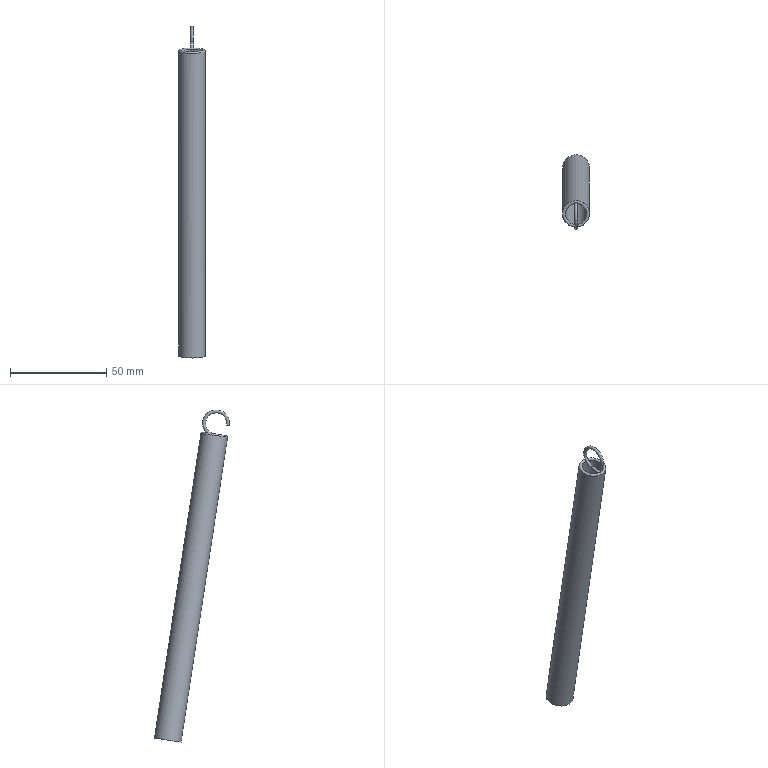Part | NX | features 1 2 | 1 solid | 7 faces | box 14 x 39.013 x 172.675 mm | volume 9539 mm3 | cylinder 3 | plane 2 | torus 2 | commonest cylinder face diameters 1.5 x1 11 x1 14 x1
STEP:
#1=CARTESIAN_POINT('',(-24.935,47.341,-652.78));
#2=VERTEX_POINT('',#1);
#3=CARTESIAN_POINT('',(-24.935,46.602,-652.906));
#4=DIRECTION('',(0.,0.1679,-0.9858));
#5=DIRECTION('',(0.,0.9858,0.1679));
#6=AXIS2_PLACEMENT_3D('',#3,#4,#5);
#7=CIRCLE('',#6,0.75);
#8=EDGE_CURVE('',#2,#2,#7,.F.);
#9=ORIENTED_EDGE('',*,*,#8,.F.);
#10=EDGE_LOOP('',(#9));
#11=FACE_BOUND('',#10,.T.);
#12=CARTESIAN_POINT('',(-24.935,46.602,-652.906));
#13=DIRECTION('',(0.,0.1679,-0.9858));
#14=DIRECTION('',(0.,-0.9858,-0.1679));
#15=AXIS2_PLACEMENT_3D('',#12,#13,#14);
#16=PLANE('',#15);
#17=ADVANCED_FACE('',(#11),#16,.T.);
#18=CARTESIAN_POINT('',(-25.685,53.704,-658.036));
#19=VERTEX_POINT('',#18);
#20=CARTESIAN_POINT('',(-24.935,53.704,-658.036));
#21=DIRECTION('',(0.,-0.9886,-0.1507));
#22=DIRECTION('',(-1.,0.,0.));
#23=AXIS2_PLACEMENT_3D('',#20,#21,#22);
#24=CIRCLE('',#23,0.75);
#25=EDGE_CURVE('',#19,#19,#24,.T.);
#26=ORIENTED_EDGE('',*,*,#25,.F.);
#27=EDGE_LOOP('',(#26));
#28=FACE_BOUND('',#27,.T.);
#29=ORIENTED_EDGE('',*,*,#8,.T.);
#30=EDGE_LOOP('',(#29));
#31=FACE_BOUND('',#30,.T.);
#32=CARTESIAN_POINT('',(-24.935,52.763,-651.857));
#33=DIRECTION('',(-1.,0.,0.));
#34=DIRECTION('',(0.,0.9886,0.1507));
#35=AXIS2_PLACEMENT_3D('',#32,#33,#34);
#36=TOROIDAL_SURFACE('',#35,6.25,0.75);
#37=ADVANCED_FACE('',(#28,#31),#36,.T.);
#38=CARTESIAN_POINT('',(-24.935,84.776,-815.458));
#39=VERTEX_POINT('',#38);
#40=CARTESIAN_POINT('',(-24.935,77.853,-816.495));
#41=DIRECTION('',(0.,-0.1481,0.989));
#42=DIRECTION('',(0.,0.989,0.1481));
#43=AXIS2_PLACEMENT_3D('',#40,#41,#42);
#44=ELLIPSE('',#43,7.,7.);
#45=EDGE_CURVE('',#39,#39,#44,.T.);
#46=ORIENTED_EDGE('',*,*,#45,.T.);
#47=EDGE_LOOP('',(#46));
#48=FACE_BOUND('',#47,.T.);
#49=CARTESIAN_POINT('',(-31.935,53.704,-658.036));
#50=VERTEX_POINT('',#49);
#51=CARTESIAN_POINT('',(-24.935,53.704,-658.036));
#52=DIRECTION('',(0.,0.1507,-0.9886));
#53=DIRECTION('',(-1.,0.,0.));
#54=AXIS2_PLACEMENT_3D('',#51,#52,#53);
#55=CIRCLE('',#54,7.);
#56=EDGE_CURVE('',#50,#50,#55,.T.);
#57=ORIENTED_EDGE('',*,*,#56,.T.);
#58=EDGE_LOOP('',(#57));
#59=FACE_BOUND('',#58,.T.);
#60=CARTESIAN_POINT('',(-24.935,59.467,-695.849));
#61=DIRECTION('',(0.,0.1507,-0.9886));
#62=DIRECTION('',(1.,0.,0.));
#63=AXIS2_PLACEMENT_3D('',#60,#61,#62);
#64=CYLINDRICAL_SURFACE('',#63,7.);
#65=ADVANCED_FACE('',(#48,#59),#64,.T.);
#66=ORIENTED_EDGE('',*,*,#56,.F.);
#67=EDGE_LOOP('',(#66));
#68=FACE_BOUND('',#67,.T.);
#69=CARTESIAN_POINT('',(-25.685,48.318,-658.856));
#70=VERTEX_POINT('',#69);
#71=CARTESIAN_POINT('',(-24.185,48.318,-658.856));
#72=VERTEX_POINT('',#71);
#73=CARTESIAN_POINT('',(-24.935,53.704,-658.036));
#74=DIRECTION('',(0.,0.1507,-0.9886));
#75=DIRECTION('',(1.,0.,0.));
#76=AXIS2_PLACEMENT_3D('',#73,#74,#75);
#77=CIRCLE('',#76,5.5);
#78=EDGE_CURVE('',#70,#72,#77,.T.);
#79=ORIENTED_EDGE('',*,*,#78,.T.);
#80=CARTESIAN_POINT('',(-24.935,47.413,-658.236));
#81=VERTEX_POINT('',#80);
#82=CARTESIAN_POINT('',(-24.185,48.318,-658.856));
#83=CARTESIAN_POINT('',(-24.185,48.281,-658.612));
#84=CARTESIAN_POINT('',(-24.428,47.944,-658.258));
#85=CARTESIAN_POINT('',(-24.763,47.582,-658.21));
#86=CARTESIAN_POINT('',(-24.935,47.413,-658.236));
#87=B_SPLINE_CURVE_WITH_KNOTS('',3,(#82,#83,#84,#85,#86),.UNSPECIFIED.,.F.,.F.,(4,1,4),(0.,0.0007272,0.001454),.UNSPECIFIED.);
#88=EDGE_CURVE('',#72,#81,#87,.T.);
#89=ORIENTED_EDGE('',*,*,#88,.T.);
#90=CARTESIAN_POINT('',(-25.685,48.318,-658.856));
#91=CARTESIAN_POINT('',(-25.685,48.281,-658.614));
#92=CARTESIAN_POINT('',(-25.44,47.942,-658.257));
#93=CARTESIAN_POINT('',(-25.107,47.583,-658.21));
#94=CARTESIAN_POINT('',(-24.935,47.413,-658.236));
#95=B_SPLINE_CURVE_WITH_KNOTS('',3,(#90,#91,#92,#93,#94),.UNSPECIFIED.,.F.,.F.,(4,1,4),(0.0004363,0.001167,0.001898),.UNSPECIFIED.);
#96=EDGE_CURVE('',#81,#70,#95,.F.);
#97=ORIENTED_EDGE('',*,*,#96,.T.);
#98=EDGE_LOOP('',(#79,#89,#97));
#99=FACE_BOUND('',#98,.T.);
#100=CARTESIAN_POINT('',(-24.935,53.704,-658.036));
#101=DIRECTION('',(0.,-0.1507,0.9886));
#102=DIRECTION('',(1.,0.,0.));
#103=AXIS2_PLACEMENT_3D('',#100,#101,#102);
#104=TOROIDAL_SURFACE('',#103,6.25,0.75);
#105=ADVANCED_FACE('',(#68,#99),#104,.T.);
#106=CARTESIAN_POINT('',(-24.185,48.318,-658.856));
#107=CARTESIAN_POINT('',(-24.185,48.378,-659.249));
#108=CARTESIAN_POINT('',(-24.934,48.383,-659.962));
#109=CARTESIAN_POINT('',(-25.685,48.378,-659.249));
#110=CARTESIAN_POINT('',(-25.685,48.318,-658.856));
#111=B_SPLINE_CURVE_WITH_KNOTS('',3,(#106,#107,#108,#109,#110),.UNSPECIFIED.,.F.,.F.,(4,1,4),(0.,0.001174,0.002347),.UNSPECIFIED.);
#112=EDGE_CURVE('',#72,#70,#111,.T.);
#113=ORIENTED_EDGE('',*,*,#112,.T.);
#114=ORIENTED_EDGE('',*,*,#96,.F.);
#115=ORIENTED_EDGE('',*,*,#88,.F.);
#116=EDGE_LOOP('',(#113,#114,#115));
#117=FACE_BOUND('',#116,.T.);
#118=ORIENTED_EDGE('',*,*,#25,.T.);
#119=EDGE_LOOP('',(#118));
#120=FACE_BOUND('',#119,.T.);
#121=CARTESIAN_POINT('',(-24.935,50.615,-658.506));
#122=DIRECTION('',(0.,-0.9886,-0.1507));
#123=DIRECTION('',(1.,0.,0.));
#124=AXIS2_PLACEMENT_3D('',#121,#122,#123);
#125=CYLINDRICAL_SURFACE('',#124,0.75);
#126=ADVANCED_FACE('',(#117,#120),#125,.T.);
#127=CARTESIAN_POINT('',(-24.935,83.292,-815.681));
#128=VERTEX_POINT('',#127);
#129=CARTESIAN_POINT('',(-24.935,77.853,-816.495));
#130=DIRECTION('',(0.,-0.1481,0.989));
#131=DIRECTION('',(0.,0.989,0.1481));
#132=AXIS2_PLACEMENT_3D('',#129,#130,#131);
#133=ELLIPSE('',#132,5.5,5.5);
#134=EDGE_CURVE('',#128,#128,#133,.F.);
#135=ORIENTED_EDGE('',*,*,#134,.T.);
#136=EDGE_LOOP('',(#135));
#137=FACE_BOUND('',#136,.T.);
#138=ORIENTED_EDGE('',*,*,#112,.F.);
#139=ORIENTED_EDGE('',*,*,#78,.F.);
#140=EDGE_LOOP('',(#138,#139));
#141=FACE_BOUND('',#140,.T.);
#142=CARTESIAN_POINT('',(-24.935,59.467,-695.849));
#143=DIRECTION('',(0.,0.1507,-0.9886));
#144=DIRECTION('',(1.,0.,0.));
#145=AXIS2_PLACEMENT_3D('',#142,#143,#144);
#146=CYLINDRICAL_SURFACE('',#145,5.5);
#147=ADVANCED_FACE('',(#137,#141),#146,.F.);
#148=ORIENTED_EDGE('',*,*,#45,.F.);
#149=EDGE_LOOP('',(#148));
#150=FACE_BOUND('',#149,.T.);
#151=ORIENTED_EDGE('',*,*,#134,.F.);
#152=EDGE_LOOP('',(#151));
#153=FACE_BOUND('',#152,.T.);
#154=CARTESIAN_POINT('',(-80.065,119.725,-810.224));
#155=DIRECTION('',(0.,-0.1481,0.989));
#156=DIRECTION('',(0.,-0.989,-0.1481));
#157=AXIS2_PLACEMENT_3D('',#154,#155,#156);
#158=PLANE('',#157);
#159=ADVANCED_FACE('',(#150,#153),#158,.F.);
#160=CLOSED_SHELL('',(#17,#37,#65,#105,#126,#147,#159));
#161=MANIFOLD_SOLID_BREP('',#160);
#162=(LENGTH_UNIT()NAMED_UNIT(*)SI_UNIT(.MILLI.,.METRE.));
#163=UNCERTAINTY_MEASURE_WITH_UNIT(LENGTH_MEASURE(0.0508),#162,'','');
#164=(NAMED_UNIT(*)PLANE_ANGLE_UNIT()SI_UNIT($,.RADIAN.));
#165=(NAMED_UNIT(*)SI_UNIT($,.STERADIAN.)SOLID_ANGLE_UNIT());
#166=(GEOMETRIC_REPRESENTATION_CONTEXT(3)GLOBAL_UNCERTAINTY_ASSIGNED_CONTEXT((#163))GLOBAL_UNIT_ASSIGNED_CONTEXT((#162,#164,#165))REPRESENTATION_CONTEXT('',''));
#167=ADVANCED_BREP_SHAPE_REPRESENTATION('',(#161),#166);